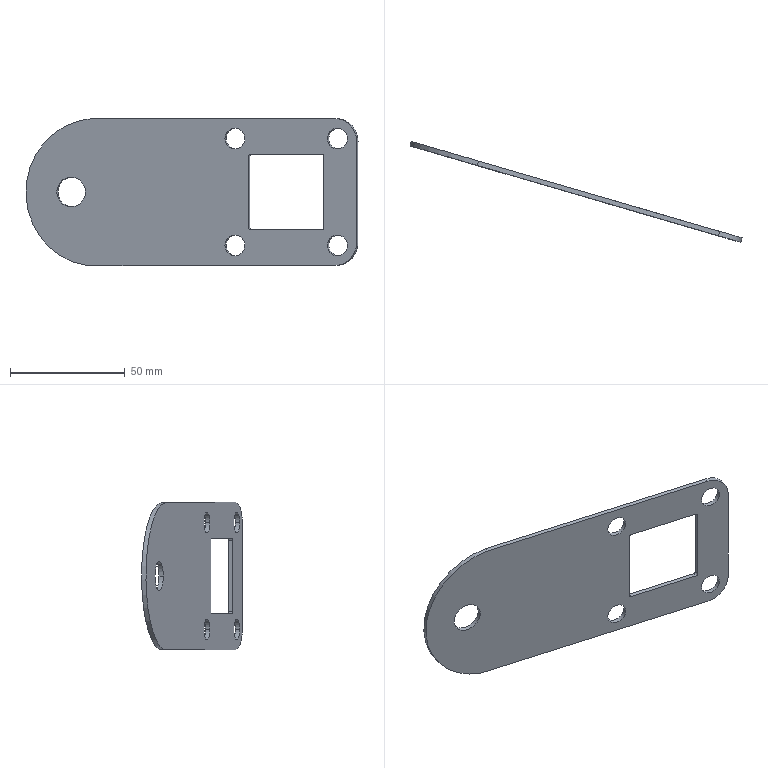Part | SolidWorks | features BaseBody 1 | 1 solid | 26 faces | box 144.562 x 43.913 x 64 mm | volume 15230 mm3 | cylinder 17 | plane 9 | commonest cylinder face diameters 9 x8 2 x4 13 x2 20 x2 64.36 x1
STEP:
#1=CARTESIAN_POINT('',(-21.256,471.051,-1.629));
#2=VERTEX_POINT('',#1);
#3=CARTESIAN_POINT('',(-29.896,473.571,-1.629));
#4=VERTEX_POINT('',#3);
#5=CARTESIAN_POINT('',(-25.576,472.311,-1.629));
#6=DIRECTION('',(0.28,0.96,0.));
#7=DIRECTION('',(-0.96,0.28,0.));
#8=AXIS2_PLACEMENT_3D('',#5,#6,#7);
#9=CIRCLE('',#8,4.5);
#10=EDGE_CURVE('',#2,#4,#9,.T.);
#11=ORIENTED_EDGE('',*,*,#10,.F.);
#12=CARTESIAN_POINT('',(-20.696,472.971,-1.629));
#13=VERTEX_POINT('',#12);
#14=CARTESIAN_POINT('',(-21.256,471.051,-1.629));
#15=DIRECTION('',(0.28,0.96,0.));
#16=VECTOR('',#15,1000.);
#17=LINE('',#14,#16);
#18=EDGE_CURVE('',#2,#13,#17,.T.);
#19=ORIENTED_EDGE('',*,*,#18,.T.);
#20=CARTESIAN_POINT('',(-29.336,475.491,-1.629));
#21=VERTEX_POINT('',#20);
#22=CARTESIAN_POINT('',(-25.016,474.231,-1.629));
#23=DIRECTION('',(-0.28,-0.96,0.));
#24=DIRECTION('',(-0.96,0.28,0.));
#25=AXIS2_PLACEMENT_3D('',#22,#23,#24);
#26=CIRCLE('',#25,4.5);
#27=EDGE_CURVE('',#21,#13,#26,.T.);
#28=ORIENTED_EDGE('',*,*,#27,.F.);
#29=CARTESIAN_POINT('',(-29.896,473.571,-1.629));
#30=DIRECTION('',(0.28,0.96,0.));
#31=VECTOR('',#30,1000.);
#32=LINE('',#29,#31);
#33=EDGE_CURVE('',#4,#21,#32,.T.);
#34=ORIENTED_EDGE('',*,*,#33,.F.);
#35=EDGE_LOOP('',(#11,#19,#28,#34));
#36=FACE_OUTER_BOUND('',#35,.T.);
#37=CARTESIAN_POINT('',(-25.576,472.311,-1.629));
#38=DIRECTION('',(0.28,0.96,0.));
#39=DIRECTION('',(-0.96,0.28,0.));
#40=AXIS2_PLACEMENT_3D('',#37,#38,#39);
#41=CYLINDRICAL_SURFACE('',#40,4.5);
#42=ADVANCED_FACE('',(#36),#41,.F.);
#43=CARTESIAN_POINT('',(23.385,458.034,-1.629));
#44=VERTEX_POINT('',#43);
#45=CARTESIAN_POINT('',(14.745,460.553,-1.629));
#46=VERTEX_POINT('',#45);
#47=CARTESIAN_POINT('',(19.065,459.293,-1.629));
#48=DIRECTION('',(0.28,0.96,0.));
#49=DIRECTION('',(-0.96,0.28,0.));
#50=AXIS2_PLACEMENT_3D('',#47,#48,#49);
#51=CIRCLE('',#50,4.5);
#52=EDGE_CURVE('',#44,#46,#51,.T.);
#53=ORIENTED_EDGE('',*,*,#52,.F.);
#54=CARTESIAN_POINT('',(23.945,459.954,-1.629));
#55=VERTEX_POINT('',#54);
#56=CARTESIAN_POINT('',(23.385,458.034,-1.629));
#57=DIRECTION('',(0.28,0.96,0.));
#58=VECTOR('',#57,1000.);
#59=LINE('',#56,#58);
#60=EDGE_CURVE('',#44,#55,#59,.T.);
#61=ORIENTED_EDGE('',*,*,#60,.T.);
#62=CARTESIAN_POINT('',(15.304,462.473,-1.629));
#63=VERTEX_POINT('',#62);
#64=CARTESIAN_POINT('',(19.624,461.213,-1.629));
#65=DIRECTION('',(-0.28,-0.96,0.));
#66=DIRECTION('',(-0.96,0.28,0.));
#67=AXIS2_PLACEMENT_3D('',#64,#65,#66);
#68=CIRCLE('',#67,4.5);
#69=EDGE_CURVE('',#63,#55,#68,.T.);
#70=ORIENTED_EDGE('',*,*,#69,.F.);
#71=CARTESIAN_POINT('',(14.745,460.553,-1.629));
#72=DIRECTION('',(0.28,0.96,0.));
#73=VECTOR('',#72,1000.);
#74=LINE('',#71,#73);
#75=EDGE_CURVE('',#46,#63,#74,.T.);
#76=ORIENTED_EDGE('',*,*,#75,.F.);
#77=EDGE_LOOP('',(#53,#61,#70,#76));
#78=FACE_OUTER_BOUND('',#77,.T.);
#79=CARTESIAN_POINT('',(19.065,459.293,-1.629));
#80=DIRECTION('',(0.28,0.96,0.));
#81=DIRECTION('',(-0.96,0.28,0.));
#82=AXIS2_PLACEMENT_3D('',#79,#80,#81);
#83=CYLINDRICAL_SURFACE('',#82,4.5);
#84=ADVANCED_FACE('',(#78),#83,.F.);
#85=CARTESIAN_POINT('',(23.385,458.034,-48.129));
#86=VERTEX_POINT('',#85);
#87=CARTESIAN_POINT('',(14.745,460.553,-48.129));
#88=VERTEX_POINT('',#87);
#89=CARTESIAN_POINT('',(19.065,459.293,-48.129));
#90=DIRECTION('',(0.28,0.96,0.));
#91=DIRECTION('',(-0.96,0.28,0.));
#92=AXIS2_PLACEMENT_3D('',#89,#90,#91);
#93=CIRCLE('',#92,4.5);
#94=EDGE_CURVE('',#86,#88,#93,.T.);
#95=ORIENTED_EDGE('',*,*,#94,.F.);
#96=CARTESIAN_POINT('',(23.945,459.954,-48.129));
#97=VERTEX_POINT('',#96);
#98=CARTESIAN_POINT('',(23.385,458.034,-48.129));
#99=DIRECTION('',(0.28,0.96,0.));
#100=VECTOR('',#99,1000.);
#101=LINE('',#98,#100);
#102=EDGE_CURVE('',#86,#97,#101,.T.);
#103=ORIENTED_EDGE('',*,*,#102,.T.);
#104=CARTESIAN_POINT('',(15.304,462.473,-48.129));
#105=VERTEX_POINT('',#104);
#106=CARTESIAN_POINT('',(19.624,461.213,-48.129));
#107=DIRECTION('',(-0.28,-0.96,0.));
#108=DIRECTION('',(-0.96,0.28,0.));
#109=AXIS2_PLACEMENT_3D('',#106,#107,#108);
#110=CIRCLE('',#109,4.5);
#111=EDGE_CURVE('',#105,#97,#110,.T.);
#112=ORIENTED_EDGE('',*,*,#111,.F.);
#113=CARTESIAN_POINT('',(14.745,460.553,-48.129));
#114=DIRECTION('',(0.28,0.96,0.));
#115=VECTOR('',#114,1000.);
#116=LINE('',#113,#115);
#117=EDGE_CURVE('',#88,#105,#116,.T.);
#118=ORIENTED_EDGE('',*,*,#117,.F.);
#119=EDGE_LOOP('',(#95,#103,#112,#118));
#120=FACE_OUTER_BOUND('',#119,.T.);
#121=CARTESIAN_POINT('',(19.065,459.293,-48.129));
#122=DIRECTION('',(0.28,0.96,0.));
#123=DIRECTION('',(-0.96,0.28,0.));
#124=AXIS2_PLACEMENT_3D('',#121,#122,#123);
#125=CYLINDRICAL_SURFACE('',#124,4.5);
#126=ADVANCED_FACE('',(#120),#125,.F.);
#127=CARTESIAN_POINT('',(-21.256,471.051,-48.129));
#128=VERTEX_POINT('',#127);
#129=CARTESIAN_POINT('',(-29.896,473.571,-48.129));
#130=VERTEX_POINT('',#129);
#131=CARTESIAN_POINT('',(-25.576,472.311,-48.129));
#132=DIRECTION('',(0.28,0.96,0.));
#133=DIRECTION('',(-0.96,0.28,0.));
#134=AXIS2_PLACEMENT_3D('',#131,#132,#133);
#135=CIRCLE('',#134,4.5);
#136=EDGE_CURVE('',#128,#130,#135,.T.);
#137=ORIENTED_EDGE('',*,*,#136,.F.);
#138=CARTESIAN_POINT('',(-20.696,472.971,-48.129));
#139=VERTEX_POINT('',#138);
#140=CARTESIAN_POINT('',(-21.256,471.051,-48.129));
#141=DIRECTION('',(0.28,0.96,0.));
#142=VECTOR('',#141,1000.);
#143=LINE('',#140,#142);
#144=EDGE_CURVE('',#128,#139,#143,.T.);
#145=ORIENTED_EDGE('',*,*,#144,.T.);
#146=CARTESIAN_POINT('',(-29.336,475.491,-48.129));
#147=VERTEX_POINT('',#146);
#148=CARTESIAN_POINT('',(-25.016,474.231,-48.129));
#149=DIRECTION('',(-0.28,-0.96,0.));
#150=DIRECTION('',(-0.96,0.28,0.));
#151=AXIS2_PLACEMENT_3D('',#148,#149,#150);
#152=CIRCLE('',#151,4.5);
#153=EDGE_CURVE('',#147,#139,#152,.T.);
#154=ORIENTED_EDGE('',*,*,#153,.F.);
#155=CARTESIAN_POINT('',(-29.896,473.571,-48.129));
#156=DIRECTION('',(0.28,0.96,0.));
#157=VECTOR('',#156,1000.);
#158=LINE('',#155,#157);
#159=EDGE_CURVE('',#130,#147,#158,.T.);
#160=ORIENTED_EDGE('',*,*,#159,.F.);
#161=EDGE_LOOP('',(#137,#145,#154,#160));
#162=FACE_OUTER_BOUND('',#161,.T.);
#163=CARTESIAN_POINT('',(-25.576,472.311,-48.129));
#164=DIRECTION('',(0.28,0.96,0.));
#165=DIRECTION('',(-0.96,0.28,0.));
#166=AXIS2_PLACEMENT_3D('',#163,#164,#165);
#167=CYLINDRICAL_SURFACE('',#166,4.5);
#168=ADVANCED_FACE('',(#162),#167,.F.);
#169=CARTESIAN_POINT('',(-102.537,496.837,-24.879));
#170=VERTEX_POINT('',#169);
#171=CARTESIAN_POINT('',(-90.057,493.198,-24.879));
#172=VERTEX_POINT('',#171);
#173=CARTESIAN_POINT('',(-96.297,495.018,-24.879));
#174=DIRECTION('',(-0.28,-0.96,0.));
#175=DIRECTION('',(0.96,-0.28,0.));
#176=AXIS2_PLACEMENT_3D('',#173,#174,#175);
#177=CIRCLE('',#176,6.5);
#178=EDGE_CURVE('',#170,#172,#177,.T.);
#179=ORIENTED_EDGE('',*,*,#178,.F.);
#180=CARTESIAN_POINT('',(-103.097,494.917,-24.879));
#181=VERTEX_POINT('',#180);
#182=CARTESIAN_POINT('',(-102.537,496.837,-24.879));
#183=DIRECTION('',(-0.28,-0.96,0.));
#184=VECTOR('',#183,1000.);
#185=LINE('',#182,#184);
#186=EDGE_CURVE('',#170,#181,#185,.T.);
#187=ORIENTED_EDGE('',*,*,#186,.T.);
#188=CARTESIAN_POINT('',(-90.617,491.278,-24.879));
#189=VERTEX_POINT('',#188);
#190=CARTESIAN_POINT('',(-96.857,493.098,-24.879));
#191=DIRECTION('',(0.28,0.96,0.));
#192=DIRECTION('',(0.96,-0.28,0.));
#193=AXIS2_PLACEMENT_3D('',#190,#191,#192);
#194=CIRCLE('',#193,6.5);
#195=EDGE_CURVE('',#189,#181,#194,.T.);
#196=ORIENTED_EDGE('',*,*,#195,.F.);
#197=CARTESIAN_POINT('',(-90.057,493.198,-24.879));
#198=DIRECTION('',(-0.28,-0.96,0.));
#199=VECTOR('',#198,1000.);
#200=LINE('',#197,#199);
#201=EDGE_CURVE('',#172,#189,#200,.T.);
#202=ORIENTED_EDGE('',*,*,#201,.F.);
#203=EDGE_LOOP('',(#179,#187,#196,#202));
#204=FACE_OUTER_BOUND('',#203,.T.);
#205=CARTESIAN_POINT('',(-96.297,495.018,-24.879));
#206=DIRECTION('',(-0.28,-0.96,0.));
#207=DIRECTION('',(0.96,-0.28,0.));
#208=AXIS2_PLACEMENT_3D('',#205,#206,#207);
#209=CYLINDRICAL_SURFACE('',#208,6.5);
#210=ADVANCED_FACE('',(#204),#209,.F.);
#211=CARTESIAN_POINT('',(-89.989,491.095,-56.879));
#212=VERTEX_POINT('',#211);
#213=CARTESIAN_POINT('',(17.865,459.643,-56.879));
#214=VERTEX_POINT('',#213);
#215=CARTESIAN_POINT('',(-44.536,477.84,-56.879));
#216=DIRECTION('',(0.96,-0.28,0.));
#217=VECTOR('',#216,1000.);
#218=LINE('',#215,#217);
#219=EDGE_CURVE('',#212,#214,#218,.T.);
#220=ORIENTED_EDGE('',*,*,#219,.T.);
#221=CARTESIAN_POINT('',(27.465,456.844,-46.879));
#222=VERTEX_POINT('',#221);
#223=CARTESIAN_POINT('',(17.865,459.643,-46.879));
#224=DIRECTION('',(-0.28,-0.96,0.));
#225=DIRECTION('',(0.96,-0.28,0.));
#226=AXIS2_PLACEMENT_3D('',#223,#224,#225);
#227=CIRCLE('',#226,10.);
#228=EDGE_CURVE('',#214,#222,#227,.T.);
#229=ORIENTED_EDGE('',*,*,#228,.T.);
#230=CARTESIAN_POINT('',(27.465,456.844,-2.879));
#231=VERTEX_POINT('',#230);
#232=CARTESIAN_POINT('',(27.465,456.844,-24.879));
#233=DIRECTION('',(0.,0.,1.));
#234=VECTOR('',#233,1000.);
#235=LINE('',#232,#234);
#236=EDGE_CURVE('',#222,#231,#235,.T.);
#237=ORIENTED_EDGE('',*,*,#236,.T.);
#238=CARTESIAN_POINT('',(17.865,459.643,7.121));
#239=VERTEX_POINT('',#238);
#240=CARTESIAN_POINT('',(17.865,459.643,-2.879));
#241=DIRECTION('',(-0.28,-0.96,0.));
#242=DIRECTION('',(0.96,-0.28,0.));
#243=AXIS2_PLACEMENT_3D('',#240,#241,#242);
#244=CIRCLE('',#243,10.);
#245=EDGE_CURVE('',#231,#239,#244,.T.);
#246=ORIENTED_EDGE('',*,*,#245,.T.);
#247=CARTESIAN_POINT('',(-87.182,490.276,7.121));
#248=VERTEX_POINT('',#247);
#249=CARTESIAN_POINT('',(-44.536,477.84,7.121));
#250=DIRECTION('',(-0.96,0.28,0.));
#251=VECTOR('',#250,1000.);
#252=LINE('',#249,#251);
#253=EDGE_CURVE('',#239,#248,#252,.T.);
#254=ORIENTED_EDGE('',*,*,#253,.T.);
#255=CARTESIAN_POINT('',(-85.644,489.828,-25.019));
#256=DIRECTION('',(-0.28,-0.96,0.));
#257=DIRECTION('',(0.96,-0.28,0.));
#258=AXIS2_PLACEMENT_3D('',#255,#256,#257);
#259=CIRCLE('',#258,32.18);
#260=EDGE_CURVE('',#248,#212,#259,.T.);
#261=ORIENTED_EDGE('',*,*,#260,.T.);
#262=EDGE_LOOP('',(#220,#229,#237,#246,#254,#261));
#263=FACE_OUTER_BOUND('',#262,.T.);
#264=CARTESIAN_POINT('',(-25.576,472.311,-1.629));
#265=DIRECTION('',(0.28,0.96,0.));
#266=DIRECTION('',(-0.96,0.28,0.));
#267=AXIS2_PLACEMENT_3D('',#264,#265,#266);
#268=CIRCLE('',#267,4.5);
#269=EDGE_CURVE('',#4,#2,#268,.T.);
#270=ORIENTED_EDGE('',*,*,#269,.T.);
#271=ORIENTED_EDGE('',*,*,#10,.T.);
#272=EDGE_LOOP('',(#270,#271));
#273=FACE_BOUND('',#272,.T.);
#274=CARTESIAN_POINT('',(19.065,459.293,-1.629));
#275=DIRECTION('',(0.28,0.96,0.));
#276=DIRECTION('',(-0.96,0.28,0.));
#277=AXIS2_PLACEMENT_3D('',#274,#275,#276);
#278=CIRCLE('',#277,4.5);
#279=EDGE_CURVE('',#46,#44,#278,.T.);
#280=ORIENTED_EDGE('',*,*,#279,.T.);
#281=ORIENTED_EDGE('',*,*,#52,.T.);
#282=EDGE_LOOP('',(#280,#281));
#283=FACE_BOUND('',#282,.T.);
#284=CARTESIAN_POINT('',(19.065,459.293,-48.129));
#285=DIRECTION('',(0.28,0.96,0.));
#286=DIRECTION('',(-0.96,0.28,0.));
#287=AXIS2_PLACEMENT_3D('',#284,#285,#286);
#288=CIRCLE('',#287,4.5);
#289=EDGE_CURVE('',#88,#86,#288,.T.);
#290=ORIENTED_EDGE('',*,*,#289,.T.);
#291=ORIENTED_EDGE('',*,*,#94,.T.);
#292=EDGE_LOOP('',(#290,#291));
#293=FACE_BOUND('',#292,.T.);
#294=CARTESIAN_POINT('',(-25.576,472.311,-48.129));
#295=DIRECTION('',(0.28,0.96,0.));
#296=DIRECTION('',(-0.96,0.28,0.));
#297=AXIS2_PLACEMENT_3D('',#294,#295,#296);
#298=CIRCLE('',#297,4.5);
#299=EDGE_CURVE('',#130,#128,#298,.T.);
#300=ORIENTED_EDGE('',*,*,#299,.T.);
#301=ORIENTED_EDGE('',*,*,#136,.T.);
#302=EDGE_LOOP('',(#300,#301));
#303=FACE_BOUND('',#302,.T.);
#304=ORIENTED_EDGE('',*,*,#195,.T.);
#305=CARTESIAN_POINT('',(-96.857,493.098,-24.879));
#306=DIRECTION('',(0.28,0.96,0.));
#307=DIRECTION('',(0.96,-0.28,0.));
#308=AXIS2_PLACEMENT_3D('',#305,#306,#307);
#309=CIRCLE('',#308,6.5);
#310=EDGE_CURVE('',#181,#189,#309,.T.);
#311=ORIENTED_EDGE('',*,*,#310,.T.);
#312=EDGE_LOOP('',(#304,#311));
#313=FACE_BOUND('',#312,.T.);
#314=CARTESIAN_POINT('',(13.065,461.043,-9.372));
#315=VERTEX_POINT('',#314);
#316=CARTESIAN_POINT('',(13.065,461.043,-40.372));
#317=VERTEX_POINT('',#316);
#318=CARTESIAN_POINT('',(13.065,461.043,-24.879));
#319=DIRECTION('',(0.,0.,-1.));
#320=VECTOR('',#319,1000.);
#321=LINE('',#318,#320);
#322=EDGE_CURVE('',#315,#317,#321,.T.);
#323=ORIENTED_EDGE('',*,*,#322,.T.);
#324=CARTESIAN_POINT('',(12.104,461.323,-41.372));
#325=VERTEX_POINT('',#324);
#326=CARTESIAN_POINT('',(12.104,461.323,-40.372));
#327=DIRECTION('',(0.28,0.96,0.));
#328=DIRECTION('',(-0.96,0.28,0.));
#329=AXIS2_PLACEMENT_3D('',#326,#327,#328);
#330=CIRCLE('',#329,1.);
#331=EDGE_CURVE('',#317,#325,#330,.T.);
#332=ORIENTED_EDGE('',*,*,#331,.T.);
#333=CARTESIAN_POINT('',(-18.616,470.282,-41.372));
#334=VERTEX_POINT('',#333);
#335=CARTESIAN_POINT('',(-44.536,477.84,-41.372));
#336=DIRECTION('',(-0.96,0.28,0.));
#337=VECTOR('',#336,1000.);
#338=LINE('',#335,#337);
#339=EDGE_CURVE('',#325,#334,#338,.T.);
#340=ORIENTED_EDGE('',*,*,#339,.T.);
#341=CARTESIAN_POINT('',(-19.576,470.562,-40.372));
#342=VERTEX_POINT('',#341);
#343=CARTESIAN_POINT('',(-18.616,470.282,-40.372));
#344=DIRECTION('',(0.28,0.96,0.));
#345=DIRECTION('',(-0.96,0.28,0.));
#346=AXIS2_PLACEMENT_3D('',#343,#344,#345);
#347=CIRCLE('',#346,1.);
#348=EDGE_CURVE('',#334,#342,#347,.T.);
#349=ORIENTED_EDGE('',*,*,#348,.T.);
#350=CARTESIAN_POINT('',(-19.576,470.562,-9.372));
#351=VERTEX_POINT('',#350);
#352=CARTESIAN_POINT('',(-19.576,470.562,-24.879));
#353=DIRECTION('',(0.,0.,1.));
#354=VECTOR('',#353,1000.);
#355=LINE('',#352,#354);
#356=EDGE_CURVE('',#342,#351,#355,.T.);
#357=ORIENTED_EDGE('',*,*,#356,.T.);
#358=CARTESIAN_POINT('',(-18.616,470.282,-8.372));
#359=VERTEX_POINT('',#358);
#360=CARTESIAN_POINT('',(-18.616,470.282,-9.372));
#361=DIRECTION('',(0.28,0.96,0.));
#362=DIRECTION('',(-0.96,0.28,0.));
#363=AXIS2_PLACEMENT_3D('',#360,#361,#362);
#364=CIRCLE('',#363,1.);
#365=EDGE_CURVE('',#351,#359,#364,.T.);
#366=ORIENTED_EDGE('',*,*,#365,.T.);
#367=CARTESIAN_POINT('',(12.104,461.323,-8.372));
#368=VERTEX_POINT('',#367);
#369=CARTESIAN_POINT('',(-44.536,477.84,-8.372));
#370=DIRECTION('',(0.96,-0.28,0.));
#371=VECTOR('',#370,1000.);
#372=LINE('',#369,#371);
#373=EDGE_CURVE('',#359,#368,#372,.T.);
#374=ORIENTED_EDGE('',*,*,#373,.T.);
#375=CARTESIAN_POINT('',(12.104,461.323,-9.372));
#376=DIRECTION('',(0.28,0.96,0.));
#377=DIRECTION('',(-0.96,0.28,0.));
#378=AXIS2_PLACEMENT_3D('',#375,#376,#377);
#379=CIRCLE('',#378,1.);
#380=EDGE_CURVE('',#368,#315,#379,.T.);
#381=ORIENTED_EDGE('',*,*,#380,.T.);
#382=EDGE_LOOP('',(#323,#332,#340,#349,#357,#366,#374,#381));
#383=FACE_BOUND('',#382,.T.);
#384=CARTESIAN_POINT('',(-44.536,477.84,-24.879));
#385=DIRECTION('',(-0.28,-0.96,0.));
#386=DIRECTION('',(0.96,-0.28,0.));
#387=AXIS2_PLACEMENT_3D('',#384,#385,#386);
#388=PLANE('',#387);
#389=ADVANCED_FACE('',(#263,#273,#283,#293,#303,#313,#383),#388,.T.);
#390=ORIENTED_EDGE('',*,*,#228,.F.);
#391=CARTESIAN_POINT('',(18.424,461.563,-56.879));
#392=VERTEX_POINT('',#391);
#393=CARTESIAN_POINT('',(18.424,461.563,-56.879));
#394=DIRECTION('',(0.28,0.96,0.));
#395=VECTOR('',#394,1000.);
#396=LINE('',#393,#395);
#397=EDGE_CURVE('',#214,#392,#396,.T.);
#398=ORIENTED_EDGE('',*,*,#397,.T.);
#399=CARTESIAN_POINT('',(28.025,458.764,-46.879));
#400=VERTEX_POINT('',#399);
#401=CARTESIAN_POINT('',(18.424,461.563,-46.879));
#402=DIRECTION('',(-0.28,-0.96,0.));
#403=DIRECTION('',(0.96,-0.28,0.));
#404=AXIS2_PLACEMENT_3D('',#401,#402,#403);
#405=CIRCLE('',#404,10.);
#406=EDGE_CURVE('',#392,#400,#405,.T.);
#407=ORIENTED_EDGE('',*,*,#406,.T.);
#408=CARTESIAN_POINT('',(28.025,458.764,-46.879));
#409=DIRECTION('',(-0.28,-0.96,0.));
#410=VECTOR('',#409,1000.);
#411=LINE('',#408,#410);
#412=EDGE_CURVE('',#400,#222,#411,.T.);
#413=ORIENTED_EDGE('',*,*,#412,.T.);
#414=EDGE_LOOP('',(#390,#398,#407,#413));
#415=FACE_OUTER_BOUND('',#414,.T.);
#416=CARTESIAN_POINT('',(18.424,461.563,-46.879));
#417=DIRECTION('',(-0.28,-0.96,0.));
#418=DIRECTION('',(0.96,-0.28,0.));
#419=AXIS2_PLACEMENT_3D('',#416,#417,#418);
#420=CYLINDRICAL_SURFACE('',#419,10.);
#421=ADVANCED_FACE('',(#415),#420,.T.);
#422=ORIENTED_EDGE('',*,*,#397,.F.);
#423=ORIENTED_EDGE('',*,*,#219,.F.);
#424=CARTESIAN_POINT('',(-89.43,493.015,-56.879));
#425=VERTEX_POINT('',#424);
#426=CARTESIAN_POINT('',(-89.43,493.015,-56.879));
#427=DIRECTION('',(-0.28,-0.96,0.));
#428=VECTOR('',#427,1000.);
#429=LINE('',#426,#428);
#430=EDGE_CURVE('',#425,#212,#429,.T.);
#431=ORIENTED_EDGE('',*,*,#430,.F.);
#432=CARTESIAN_POINT('',(18.424,461.563,-56.879));
#433=DIRECTION('',(-0.96,0.28,0.));
#434=VECTOR('',#433,1000.);
#435=LINE('',#432,#434);
#436=EDGE_CURVE('',#392,#425,#435,.T.);
#437=ORIENTED_EDGE('',*,*,#436,.F.);
#438=EDGE_LOOP('',(#422,#423,#431,#437));
#439=FACE_OUTER_BOUND('',#438,.T.);
#440=CARTESIAN_POINT('',(28.025,458.764,-56.879));
#441=DIRECTION('',(0.,0.,1.));
#442=DIRECTION('',(1.,0.,0.));
#443=AXIS2_PLACEMENT_3D('',#440,#441,#442);
#444=PLANE('',#443);
#445=ADVANCED_FACE('',(#439),#444,.F.);
#446=CARTESIAN_POINT('',(-86.622,492.196,7.121));
#447=VERTEX_POINT('',#446);
#448=CARTESIAN_POINT('',(-85.084,491.748,-25.019));
#449=DIRECTION('',(-0.28,-0.96,0.));
#450=DIRECTION('',(0.96,-0.28,0.));
#451=AXIS2_PLACEMENT_3D('',#448,#449,#450);
#452=CIRCLE('',#451,32.18);
#453=EDGE_CURVE('',#447,#425,#452,.T.);
#454=ORIENTED_EDGE('',*,*,#453,.T.);
#455=ORIENTED_EDGE('',*,*,#430,.T.);
#456=ORIENTED_EDGE('',*,*,#260,.F.);
#457=CARTESIAN_POINT('',(-86.622,492.196,7.121));
#458=DIRECTION('',(0.28,0.96,0.));
#459=VECTOR('',#458,1000.);
#460=LINE('',#457,#459);
#461=EDGE_CURVE('',#248,#447,#460,.T.);
#462=ORIENTED_EDGE('',*,*,#461,.T.);
#463=EDGE_LOOP('',(#454,#455,#456,#462));
#464=FACE_OUTER_BOUND('',#463,.T.);
#465=CARTESIAN_POINT('',(-85.084,491.748,-25.019));
#466=DIRECTION('',(-0.28,-0.96,0.));
#467=DIRECTION('',(0.96,-0.28,0.));
#468=AXIS2_PLACEMENT_3D('',#465,#466,#467);
#469=CYLINDRICAL_SURFACE('',#468,32.18);
#470=ADVANCED_FACE('',(#464),#469,.T.);
#471=CARTESIAN_POINT('',(18.424,461.563,7.121));
#472=VERTEX_POINT('',#471);
#473=CARTESIAN_POINT('',(18.424,461.563,7.121));
#474=DIRECTION('',(-0.28,-0.96,0.));
#475=VECTOR('',#474,1000.);
#476=LINE('',#473,#475);
#477=EDGE_CURVE('',#472,#239,#476,.T.);
#478=ORIENTED_EDGE('',*,*,#477,.F.);
#479=CARTESIAN_POINT('',(-86.622,492.196,7.121));
#480=DIRECTION('',(0.96,-0.28,0.));
#481=VECTOR('',#480,1000.);
#482=LINE('',#479,#481);
#483=EDGE_CURVE('',#447,#472,#482,.T.);
#484=ORIENTED_EDGE('',*,*,#483,.F.);
#485=ORIENTED_EDGE('',*,*,#461,.F.);
#486=ORIENTED_EDGE('',*,*,#253,.F.);
#487=EDGE_LOOP('',(#478,#484,#485,#486));
#488=FACE_OUTER_BOUND('',#487,.T.);
#489=CARTESIAN_POINT('',(28.025,458.764,7.121));
#490=DIRECTION('',(0.,0.,-1.));
#491=DIRECTION('',(-1.,0.,0.));
#492=AXIS2_PLACEMENT_3D('',#489,#490,#491);
#493=PLANE('',#492);
#494=ADVANCED_FACE('',(#488),#493,.F.);
#495=ORIENTED_EDGE('',*,*,#245,.F.);
#496=CARTESIAN_POINT('',(28.025,458.764,-2.879));
#497=VERTEX_POINT('',#496);
#498=CARTESIAN_POINT('',(28.025,458.764,-2.879));
#499=DIRECTION('',(0.28,0.96,0.));
#500=VECTOR('',#499,1000.);
#501=LINE('',#498,#500);
#502=EDGE_CURVE('',#231,#497,#501,.T.);
#503=ORIENTED_EDGE('',*,*,#502,.T.);
#504=CARTESIAN_POINT('',(18.424,461.563,-2.879));
#505=DIRECTION('',(-0.28,-0.96,0.));
#506=DIRECTION('',(0.96,-0.28,0.));
#507=AXIS2_PLACEMENT_3D('',#504,#505,#506);
#508=CIRCLE('',#507,10.);
#509=EDGE_CURVE('',#497,#472,#508,.T.);
#510=ORIENTED_EDGE('',*,*,#509,.T.);
#511=ORIENTED_EDGE('',*,*,#477,.T.);
#512=EDGE_LOOP('',(#495,#503,#510,#511));
#513=FACE_OUTER_BOUND('',#512,.T.);
#514=CARTESIAN_POINT('',(18.424,461.563,-2.879));
#515=DIRECTION('',(-0.28,-0.96,0.));
#516=DIRECTION('',(0.96,-0.28,0.));
#517=AXIS2_PLACEMENT_3D('',#514,#515,#516);
#518=CYLINDRICAL_SURFACE('',#517,10.);
#519=ADVANCED_FACE('',(#513),#518,.T.);
#520=ORIENTED_EDGE('',*,*,#502,.F.);
#521=ORIENTED_EDGE('',*,*,#236,.F.);
#522=ORIENTED_EDGE('',*,*,#412,.F.);
#523=CARTESIAN_POINT('',(28.025,458.764,7.121));
#524=DIRECTION('',(0.,0.,-1.));
#525=VECTOR('',#524,1000.);
#526=LINE('',#523,#525);
#527=EDGE_CURVE('',#497,#400,#526,.T.);
#528=ORIENTED_EDGE('',*,*,#527,.F.);
#529=EDGE_LOOP('',(#520,#521,#522,#528));
#530=FACE_OUTER_BOUND('',#529,.T.);
#531=CARTESIAN_POINT('',(28.025,458.764,7.121));
#532=DIRECTION('',(-0.96,0.28,0.));
#533=DIRECTION('',(-0.28,-0.96,0.));
#534=AXIS2_PLACEMENT_3D('',#531,#532,#533);
#535=PLANE('',#534);
#536=ADVANCED_FACE('',(#530),#535,.F.);
#537=ORIENTED_EDGE('',*,*,#18,.F.);
#538=ORIENTED_EDGE('',*,*,#269,.F.);
#539=ORIENTED_EDGE('',*,*,#33,.T.);
#540=CARTESIAN_POINT('',(-25.016,474.231,-1.629));
#541=DIRECTION('',(-0.28,-0.96,0.));
#542=DIRECTION('',(-0.96,0.28,0.));
#543=AXIS2_PLACEMENT_3D('',#540,#541,#542);
#544=CIRCLE('',#543,4.5);
#545=EDGE_CURVE('',#13,#21,#544,.T.);
#546=ORIENTED_EDGE('',*,*,#545,.F.);
#547=EDGE_LOOP('',(#537,#538,#539,#546));
#548=FACE_OUTER_BOUND('',#547,.T.);
#549=CARTESIAN_POINT('',(-25.576,472.311,-1.629));
#550=DIRECTION('',(0.28,0.96,0.));
#551=DIRECTION('',(-0.96,0.28,0.));
#552=AXIS2_PLACEMENT_3D('',#549,#550,#551);
#553=CYLINDRICAL_SURFACE('',#552,4.5);
#554=ADVANCED_FACE('',(#548),#553,.F.);
#555=ORIENTED_EDGE('',*,*,#60,.F.);
#556=ORIENTED_EDGE('',*,*,#279,.F.);
#557=ORIENTED_EDGE('',*,*,#75,.T.);
#558=CARTESIAN_POINT('',(19.624,461.213,-1.629));
#559=DIRECTION('',(-0.28,-0.96,0.));
#560=DIRECTION('',(-0.96,0.28,0.));
#561=AXIS2_PLACEMENT_3D('',#558,#559,#560);
#562=CIRCLE('',#561,4.5);
#563=EDGE_CURVE('',#55,#63,#562,.T.);
#564=ORIENTED_EDGE('',*,*,#563,.F.);
#565=EDGE_LOOP('',(#555,#556,#557,#564));
#566=FACE_OUTER_BOUND('',#565,.T.);
#567=CARTESIAN_POINT('',(19.065,459.293,-1.629));
#568=DIRECTION('',(0.28,0.96,0.));
#569=DIRECTION('',(-0.96,0.28,0.));
#570=AXIS2_PLACEMENT_3D('',#567,#568,#569);
#571=CYLINDRICAL_SURFACE('',#570,4.5);
#572=ADVANCED_FACE('',(#566),#571,.F.);
#573=ORIENTED_EDGE('',*,*,#102,.F.);
#574=ORIENTED_EDGE('',*,*,#289,.F.);
#575=ORIENTED_EDGE('',*,*,#117,.T.);
#576=CARTESIAN_POINT('',(19.624,461.213,-48.129));
#577=DIRECTION('',(-0.28,-0.96,0.));
#578=DIRECTION('',(-0.96,0.28,0.));
#579=AXIS2_PLACEMENT_3D('',#576,#577,#578);
#580=CIRCLE('',#579,4.5);
#581=EDGE_CURVE('',#97,#105,#580,.T.);
#582=ORIENTED_EDGE('',*,*,#581,.F.);
#583=EDGE_LOOP('',(#573,#574,#575,#582));
#584=FACE_OUTER_BOUND('',#583,.T.);
#585=CARTESIAN_POINT('',(19.065,459.293,-48.129));
#586=DIRECTION('',(0.28,0.96,0.));
#587=DIRECTION('',(-0.96,0.28,0.));
#588=AXIS2_PLACEMENT_3D('',#585,#586,#587);
#589=CYLINDRICAL_SURFACE('',#588,4.5);
#590=ADVANCED_FACE('',(#584),#589,.F.);
#591=ORIENTED_EDGE('',*,*,#144,.F.);
#592=ORIENTED_EDGE('',*,*,#299,.F.);
#593=ORIENTED_EDGE('',*,*,#159,.T.);
#594=CARTESIAN_POINT('',(-25.016,474.231,-48.129));
#595=DIRECTION('',(-0.28,-0.96,0.));
#596=DIRECTION('',(-0.96,0.28,0.));
#597=AXIS2_PLACEMENT_3D('',#594,#595,#596);
#598=CIRCLE('',#597,4.5);
#599=EDGE_CURVE('',#139,#147,#598,.T.);
#600=ORIENTED_EDGE('',*,*,#599,.F.);
#601=EDGE_LOOP('',(#591,#592,#593,#600));
#602=FACE_OUTER_BOUND('',#601,.T.);
#603=CARTESIAN_POINT('',(-25.576,472.311,-48.129));
#604=DIRECTION('',(0.28,0.96,0.));
#605=DIRECTION('',(-0.96,0.28,0.));
#606=AXIS2_PLACEMENT_3D('',#603,#604,#605);
#607=CYLINDRICAL_SURFACE('',#606,4.5);
#608=ADVANCED_FACE('',(#602),#607,.F.);
#609=ORIENTED_EDGE('',*,*,#186,.F.);
#610=CARTESIAN_POINT('',(-96.297,495.018,-24.879));
#611=DIRECTION('',(-0.28,-0.96,0.));
#612=DIRECTION('',(0.96,-0.28,0.));
#613=AXIS2_PLACEMENT_3D('',#610,#611,#612);
#614=CIRCLE('',#613,6.5);
#615=EDGE_CURVE('',#172,#170,#614,.T.);
#616=ORIENTED_EDGE('',*,*,#615,.F.);
#617=ORIENTED_EDGE('',*,*,#201,.T.);
#618=ORIENTED_EDGE('',*,*,#310,.F.);
#619=EDGE_LOOP('',(#609,#616,#617,#618));
#620=FACE_OUTER_BOUND('',#619,.T.);
#621=CARTESIAN_POINT('',(-96.297,495.018,-24.879));
#622=DIRECTION('',(-0.28,-0.96,0.));
#623=DIRECTION('',(0.96,-0.28,0.));
#624=AXIS2_PLACEMENT_3D('',#621,#622,#623);
#625=CYLINDRICAL_SURFACE('',#624,6.5);
#626=ADVANCED_FACE('',(#620),#625,.F.);
#627=CARTESIAN_POINT('',(13.624,462.963,-40.372));
#628=VERTEX_POINT('',#627);
#629=CARTESIAN_POINT('',(13.624,462.963,-40.372));
#630=DIRECTION('',(0.28,0.96,0.));
#631=VECTOR('',#630,1000.);
#632=LINE('',#629,#631);
#633=EDGE_CURVE('',#317,#628,#632,.T.);
#634=ORIENTED_EDGE('',*,*,#633,.F.);
#635=ORIENTED_EDGE('',*,*,#322,.F.);
#636=CARTESIAN_POINT('',(13.624,462.963,-9.372));
#637=VERTEX_POINT('',#636);
#638=CARTESIAN_POINT('',(13.624,462.963,-9.372));
#639=DIRECTION('',(-0.28,-0.96,0.));
#640=VECTOR('',#639,1000.);
#641=LINE('',#638,#640);
#642=EDGE_CURVE('',#637,#315,#641,.T.);
#643=ORIENTED_EDGE('',*,*,#642,.F.);
#644=CARTESIAN_POINT('',(13.624,462.963,-8.372));
#645=DIRECTION('',(0.,0.,1.));
#646=VECTOR('',#645,1000.);
#647=LINE('',#644,#646);
#648=EDGE_CURVE('',#628,#637,#647,.T.);
#649=ORIENTED_EDGE('',*,*,#648,.F.);
#650=EDGE_LOOP('',(#634,#635,#643,#649));
#651=FACE_OUTER_BOUND('',#650,.T.);
#652=CARTESIAN_POINT('',(13.624,462.963,-8.372));
#653=DIRECTION('',(0.96,-0.28,0.));
#654=DIRECTION('',(0.28,0.96,0.));
#655=AXIS2_PLACEMENT_3D('',#652,#653,#654);
#656=PLANE('',#655);
#657=ADVANCED_FACE('',(#651),#656,.F.);
#658=CARTESIAN_POINT('',(-18.056,472.202,-8.372));
#659=VERTEX_POINT('',#658);
#660=CARTESIAN_POINT('',(-18.056,472.202,-8.372));
#661=DIRECTION('',(-0.28,-0.96,0.));
#662=VECTOR('',#661,1000.);
#663=LINE('',#660,#662);
#664=EDGE_CURVE('',#659,#359,#663,.T.);
#665=ORIENTED_EDGE('',*,*,#664,.F.);
#666=CARTESIAN_POINT('',(12.664,463.243,-8.372));
#667=VERTEX_POINT('',#666);
#668=CARTESIAN_POINT('',(12.664,463.243,-8.372));
#669=DIRECTION('',(-0.96,0.28,0.));
#670=VECTOR('',#669,1000.);
#671=LINE('',#668,#670);
#672=EDGE_CURVE('',#667,#659,#671,.T.);
#673=ORIENTED_EDGE('',*,*,#672,.F.);
#674=CARTESIAN_POINT('',(12.104,461.323,-8.372));
#675=DIRECTION('',(0.28,0.96,0.));
#676=VECTOR('',#675,1000.);
#677=LINE('',#674,#676);
#678=EDGE_CURVE('',#368,#667,#677,.T.);
#679=ORIENTED_EDGE('',*,*,#678,.F.);
#680=ORIENTED_EDGE('',*,*,#373,.F.);
#681=EDGE_LOOP('',(#665,#673,#679,#680));
#682=FACE_OUTER_BOUND('',#681,.T.);
#683=CARTESIAN_POINT('',(13.624,462.963,-8.372));
#684=DIRECTION('',(0.,0.,1.));
#685=DIRECTION('',(1.,0.,0.));
#686=AXIS2_PLACEMENT_3D('',#683,#684,#685);
#687=PLANE('',#686);
#688=ADVANCED_FACE('',(#682),#687,.F.);
#689=CARTESIAN_POINT('',(-19.016,472.482,-9.372));
#690=VERTEX_POINT('',#689);
#691=CARTESIAN_POINT('',(-19.016,472.482,-9.372));
#692=DIRECTION('',(0.28,0.96,0.));
#693=VECTOR('',#692,1000.);
#694=LINE('',#691,#693);
#695=EDGE_CURVE('',#351,#690,#694,.T.);
#696=ORIENTED_EDGE('',*,*,#695,.F.);
#697=ORIENTED_EDGE('',*,*,#356,.F.);
#698=CARTESIAN_POINT('',(-19.016,472.482,-40.372));
#699=VERTEX_POINT('',#698);
#700=CARTESIAN_POINT('',(-19.016,472.482,-40.372));
#701=DIRECTION('',(-0.28,-0.96,0.));
#702=VECTOR('',#701,1000.);
#703=LINE('',#700,#702);
#704=EDGE_CURVE('',#699,#342,#703,.T.);
#705=ORIENTED_EDGE('',*,*,#704,.F.);
#706=CARTESIAN_POINT('',(-19.016,472.482,-8.372));
#707=DIRECTION('',(0.,0.,-1.));
#708=VECTOR('',#707,1000.);
#709=LINE('',#706,#708);
#710=EDGE_CURVE('',#690,#699,#709,.T.);
#711=ORIENTED_EDGE('',*,*,#710,.F.);
#712=EDGE_LOOP('',(#696,#697,#705,#711));
#713=FACE_OUTER_BOUND('',#712,.T.);
#714=CARTESIAN_POINT('',(-19.016,472.482,-8.372));
#715=DIRECTION('',(-0.96,0.28,0.));
#716=DIRECTION('',(-0.28,-0.96,0.));
#717=AXIS2_PLACEMENT_3D('',#714,#715,#716);
#718=PLANE('',#717);
#719=ADVANCED_FACE('',(#713),#718,.F.);
#720=CARTESIAN_POINT('',(-18.056,472.202,-41.372));
#721=VERTEX_POINT('',#720);
#722=CARTESIAN_POINT('',(-18.616,470.282,-41.372));
#723=DIRECTION('',(0.28,0.96,0.));
#724=VECTOR('',#723,1000.);
#725=LINE('',#722,#724);
#726=EDGE_CURVE('',#334,#721,#725,.T.);
#727=ORIENTED_EDGE('',*,*,#726,.F.);
#728=ORIENTED_EDGE('',*,*,#339,.F.);
#729=CARTESIAN_POINT('',(12.664,463.243,-41.372));
#730=VERTEX_POINT('',#729);
#731=CARTESIAN_POINT('',(12.664,463.243,-41.372));
#732=DIRECTION('',(-0.28,-0.96,0.));
#733=VECTOR('',#732,1000.);
#734=LINE('',#731,#733);
#735=EDGE_CURVE('',#730,#325,#734,.T.);
#736=ORIENTED_EDGE('',*,*,#735,.F.);
#737=CARTESIAN_POINT('',(-18.056,472.202,-41.372));
#738=DIRECTION('',(0.96,-0.28,0.));
#739=VECTOR('',#738,1000.);
#740=LINE('',#737,#739);
#741=EDGE_CURVE('',#721,#730,#740,.T.);
#742=ORIENTED_EDGE('',*,*,#741,.F.);
#743=EDGE_LOOP('',(#727,#728,#736,#742));
#744=FACE_OUTER_BOUND('',#743,.T.);
#745=CARTESIAN_POINT('',(13.624,462.963,-41.372));
#746=DIRECTION('',(0.,0.,-1.));
#747=DIRECTION('',(-1.,0.,0.));
#748=AXIS2_PLACEMENT_3D('',#745,#746,#747);
#749=PLANE('',#748);
#750=ADVANCED_FACE('',(#744),#749,.F.);
#751=ORIENTED_EDGE('',*,*,#509,.F.);
#752=ORIENTED_EDGE('',*,*,#527,.T.);
#753=ORIENTED_EDGE('',*,*,#406,.F.);
#754=ORIENTED_EDGE('',*,*,#436,.T.);
#755=ORIENTED_EDGE('',*,*,#453,.F.);
#756=ORIENTED_EDGE('',*,*,#483,.T.);
#757=EDGE_LOOP('',(#751,#752,#753,#754,#755,#756));
#758=FACE_OUTER_BOUND('',#757,.T.);
#759=ORIENTED_EDGE('',*,*,#27,.T.);
#760=ORIENTED_EDGE('',*,*,#545,.T.);
#761=EDGE_LOOP('',(#759,#760));
#762=FACE_BOUND('',#761,.T.);
#763=ORIENTED_EDGE('',*,*,#69,.T.);
#764=ORIENTED_EDGE('',*,*,#563,.T.);
#765=EDGE_LOOP('',(#763,#764));
#766=FACE_BOUND('',#765,.T.);
#767=ORIENTED_EDGE('',*,*,#111,.T.);
#768=ORIENTED_EDGE('',*,*,#581,.T.);
#769=EDGE_LOOP('',(#767,#768));
#770=FACE_BOUND('',#769,.T.);
#771=ORIENTED_EDGE('',*,*,#153,.T.);
#772=ORIENTED_EDGE('',*,*,#599,.T.);
#773=EDGE_LOOP('',(#771,#772));
#774=FACE_BOUND('',#773,.T.);
#775=ORIENTED_EDGE('',*,*,#615,.T.);
#776=ORIENTED_EDGE('',*,*,#178,.T.);
#777=EDGE_LOOP('',(#775,#776));
#778=FACE_BOUND('',#777,.T.);
#779=CARTESIAN_POINT('',(-18.056,472.202,-9.372));
#780=DIRECTION('',(0.28,0.96,0.));
#781=DIRECTION('',(-0.96,0.28,0.));
#782=AXIS2_PLACEMENT_3D('',#779,#780,#781);
#783=CIRCLE('',#782,1.);
#784=EDGE_CURVE('',#690,#659,#783,.T.);
#785=ORIENTED_EDGE('',*,*,#784,.F.);
#786=ORIENTED_EDGE('',*,*,#710,.T.);
#787=CARTESIAN_POINT('',(-18.056,472.202,-40.372));
#788=DIRECTION('',(0.28,0.96,0.));
#789=DIRECTION('',(-0.96,0.28,0.));
#790=AXIS2_PLACEMENT_3D('',#787,#788,#789);
#791=CIRCLE('',#790,1.);
#792=EDGE_CURVE('',#721,#699,#791,.T.);
#793=ORIENTED_EDGE('',*,*,#792,.F.);
#794=ORIENTED_EDGE('',*,*,#741,.T.);
#795=CARTESIAN_POINT('',(12.664,463.243,-40.372));
#796=DIRECTION('',(0.28,0.96,0.));
#797=DIRECTION('',(-0.96,0.28,0.));
#798=AXIS2_PLACEMENT_3D('',#795,#796,#797);
#799=CIRCLE('',#798,1.);
#800=EDGE_CURVE('',#628,#730,#799,.T.);
#801=ORIENTED_EDGE('',*,*,#800,.F.);
#802=ORIENTED_EDGE('',*,*,#648,.T.);
#803=CARTESIAN_POINT('',(12.664,463.243,-9.372));
#804=DIRECTION('',(0.28,0.96,0.));
#805=DIRECTION('',(-0.96,0.28,0.));
#806=AXIS2_PLACEMENT_3D('',#803,#804,#805);
#807=CIRCLE('',#806,1.);
#808=EDGE_CURVE('',#667,#637,#807,.T.);
#809=ORIENTED_EDGE('',*,*,#808,.F.);
#810=ORIENTED_EDGE('',*,*,#672,.T.);
#811=EDGE_LOOP('',(#785,#786,#793,#794,#801,#802,#809,#810));
#812=FACE_BOUND('',#811,.T.);
#813=CARTESIAN_POINT('',(-43.976,479.76,-24.879));
#814=DIRECTION('',(-0.28,-0.96,0.));
#815=DIRECTION('',(0.96,-0.28,0.));
#816=AXIS2_PLACEMENT_3D('',#813,#814,#815);
#817=PLANE('',#816);
#818=ADVANCED_FACE('',(#758,#762,#766,#770,#774,#778,#812),#817,.F.);
#819=ORIENTED_EDGE('',*,*,#735,.T.);
#820=ORIENTED_EDGE('',*,*,#331,.F.);
#821=ORIENTED_EDGE('',*,*,#633,.T.);
#822=ORIENTED_EDGE('',*,*,#800,.T.);
#823=EDGE_LOOP('',(#819,#820,#821,#822));
#824=FACE_OUTER_BOUND('',#823,.T.);
#825=CARTESIAN_POINT('',(12.664,463.243,-40.372));
#826=DIRECTION('',(0.28,0.96,0.));
#827=DIRECTION('',(-0.96,0.28,0.));
#828=AXIS2_PLACEMENT_3D('',#825,#826,#827);
#829=CYLINDRICAL_SURFACE('',#828,1.);
#830=ADVANCED_FACE('',(#824),#829,.F.);
#831=ORIENTED_EDGE('',*,*,#642,.T.);
#832=ORIENTED_EDGE('',*,*,#380,.F.);
#833=ORIENTED_EDGE('',*,*,#678,.T.);
#834=ORIENTED_EDGE('',*,*,#808,.T.);
#835=EDGE_LOOP('',(#831,#832,#833,#834));
#836=FACE_OUTER_BOUND('',#835,.T.);
#837=CARTESIAN_POINT('',(12.664,463.243,-9.372));
#838=DIRECTION('',(0.28,0.96,0.));
#839=DIRECTION('',(-0.96,0.28,0.));
#840=AXIS2_PLACEMENT_3D('',#837,#838,#839);
#841=CYLINDRICAL_SURFACE('',#840,1.);
#842=ADVANCED_FACE('',(#836),#841,.F.);
#843=ORIENTED_EDGE('',*,*,#664,.T.);
#844=ORIENTED_EDGE('',*,*,#365,.F.);
#845=ORIENTED_EDGE('',*,*,#695,.T.);
#846=ORIENTED_EDGE('',*,*,#784,.T.);
#847=EDGE_LOOP('',(#843,#844,#845,#846));
#848=FACE_OUTER_BOUND('',#847,.T.);
#849=CARTESIAN_POINT('',(-18.056,472.202,-9.372));
#850=DIRECTION('',(0.28,0.96,0.));
#851=DIRECTION('',(-0.96,0.28,0.));
#852=AXIS2_PLACEMENT_3D('',#849,#850,#851);
#853=CYLINDRICAL_SURFACE('',#852,1.);
#854=ADVANCED_FACE('',(#848),#853,.F.);
#855=ORIENTED_EDGE('',*,*,#704,.T.);
#856=ORIENTED_EDGE('',*,*,#348,.F.);
#857=ORIENTED_EDGE('',*,*,#726,.T.);
#858=ORIENTED_EDGE('',*,*,#792,.T.);
#859=EDGE_LOOP('',(#855,#856,#857,#858));
#860=FACE_OUTER_BOUND('',#859,.T.);
#861=CARTESIAN_POINT('',(-18.056,472.202,-40.372));
#862=DIRECTION('',(0.28,0.96,0.));
#863=DIRECTION('',(-0.96,0.28,0.));
#864=AXIS2_PLACEMENT_3D('',#861,#862,#863);
#865=CYLINDRICAL_SURFACE('',#864,1.);
#866=ADVANCED_FACE('',(#860),#865,.F.);
#867=CLOSED_SHELL('',(#42,#84,#126,#168,#210,#389,#421,#445,#470,#494,#519,#536,#554,#572,#590,#608,#626,#657,#688,#719,#750,#818,#830,#842,#854,#866));
#868=MANIFOLD_SOLID_BREP('',#867);
#869=CARTESIAN_POINT('',(0.,0.,0.));
#870=DIRECTION('',(0.,0.,1.));
#871=DIRECTION('',(1.,0.,0.));
#872=AXIS2_PLACEMENT_3D('',#869,#870,#871);
#873=(LENGTH_UNIT()NAMED_UNIT(*)SI_UNIT(.MILLI.,.METRE.));
#874=UNCERTAINTY_MEASURE_WITH_UNIT(LENGTH_MEASURE(0.00001),#873,'','');
#875=(NAMED_UNIT(*)PLANE_ANGLE_UNIT()SI_UNIT($,.RADIAN.));
#876=(NAMED_UNIT(*)SI_UNIT($,.STERADIAN.)SOLID_ANGLE_UNIT());
#877=(GEOMETRIC_REPRESENTATION_CONTEXT(3)GLOBAL_UNCERTAINTY_ASSIGNED_CONTEXT((#874))GLOBAL_UNIT_ASSIGNED_CONTEXT((#873,#875,#876))REPRESENTATION_CONTEXT('',''));
#878=ADVANCED_BREP_SHAPE_REPRESENTATION('',(#868,#872),#877);